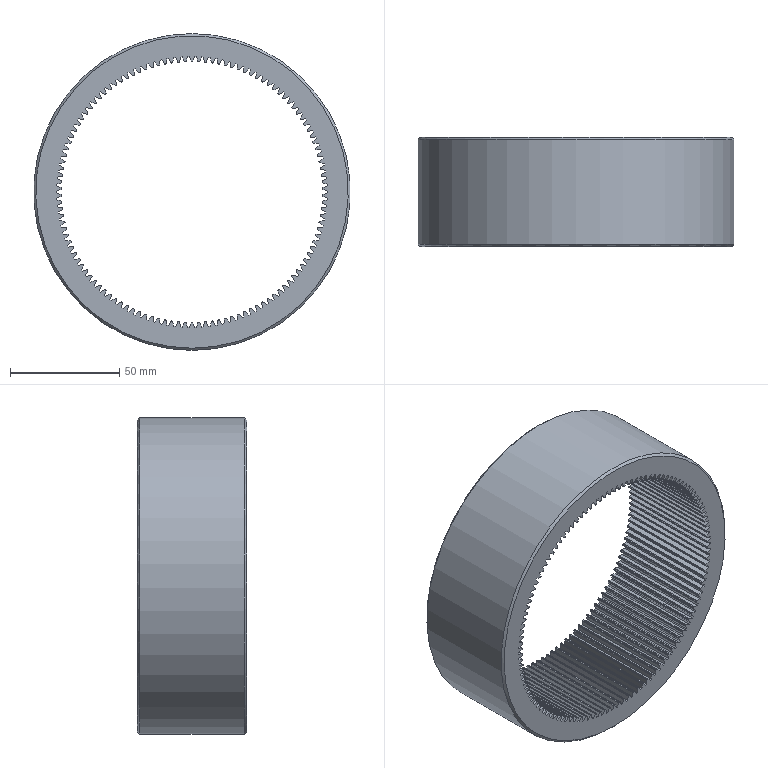Part | NX | features BREP 122, META 122, DATUM_CSYS 3, SKETCH 2, CHAMFER 1, CYLINDER 1, EXTRUDE 1, FSET 1, SUBTRACT 1 | 1 solid | 737 faces | box 145 x 50 x 145 mm | volume 241883 mm3 | spline 610 | cylinder 123 | plane 2 | cone 2 | commonest cylinder face diameters 119.5 x122 145 x1